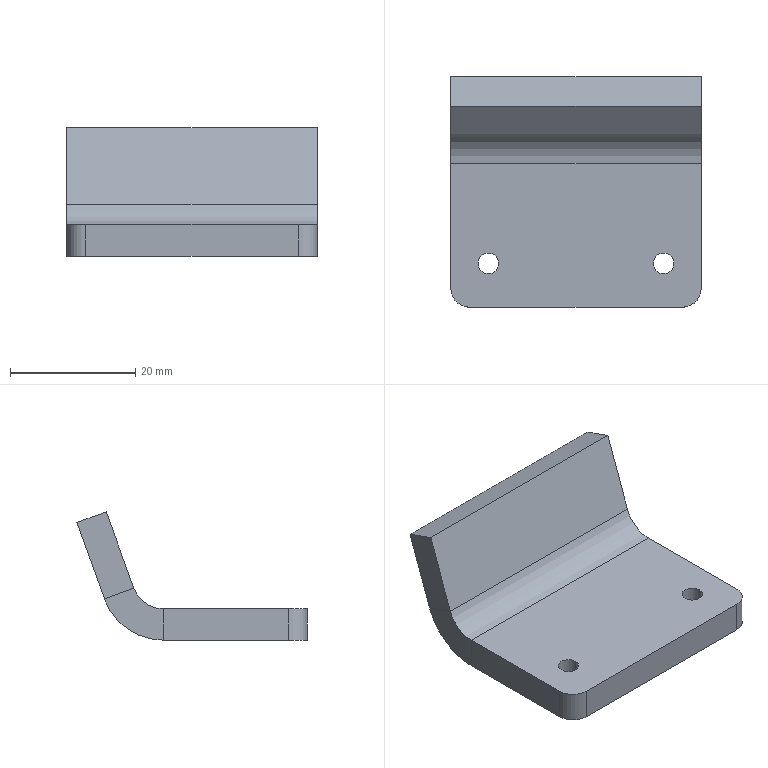Part | SolidWorks | features Fillet 1, FlatPattern 1, HoleWzd 1, ICE 1, SMBaseFlange 1, SheetMetal 1 | 1 solid | 20 faces | box 40 x 36.8 x 20.501 mm | volume 8922 mm3 | plane 12 | cylinder 8 | commonest cylinder face diameters 3.3 x4 6 x2 10 x1 20 x1
STEP:
#1=CARTESIAN_POINT('',(4.35,7.,0.));
#2=VERTEX_POINT('',#1);
#3=CARTESIAN_POINT('',(7.65,7.,0.));
#4=VERTEX_POINT('',#3);
#5=CARTESIAN_POINT('',(6.,7.,0.));
#6=DIRECTION('',(0.,0.,1.));
#7=DIRECTION('',(1.,0.,0.));
#8=AXIS2_PLACEMENT_3D('',#5,#6,#7);
#9=CIRCLE('',#8,1.65);
#10=EDGE_CURVE('',#2,#4,#9,.T.);
#11=ORIENTED_EDGE('',*,*,#10,.F.);
#12=CARTESIAN_POINT('',(4.35,7.,5.));
#13=VERTEX_POINT('',#12);
#14=CARTESIAN_POINT('',(4.35,7.,5.));
#15=DIRECTION('',(0.,0.,1.));
#16=VECTOR('',#15,1000.);
#17=LINE('',#14,#16);
#18=EDGE_CURVE('',#2,#13,#17,.T.);
#19=ORIENTED_EDGE('',*,*,#18,.T.);
#20=CARTESIAN_POINT('',(7.65,7.,5.));
#21=VERTEX_POINT('',#20);
#22=CARTESIAN_POINT('',(6.,7.,5.));
#23=DIRECTION('',(0.,0.,1.));
#24=DIRECTION('',(1.,0.,0.));
#25=AXIS2_PLACEMENT_3D('',#22,#23,#24);
#26=CIRCLE('',#25,1.65);
#27=EDGE_CURVE('',#13,#21,#26,.T.);
#28=ORIENTED_EDGE('',*,*,#27,.T.);
#29=CARTESIAN_POINT('',(7.65,7.,5.));
#30=DIRECTION('',(0.,0.,1.));
#31=VECTOR('',#30,1000.);
#32=LINE('',#29,#31);
#33=EDGE_CURVE('',#4,#21,#32,.T.);
#34=ORIENTED_EDGE('',*,*,#33,.F.);
#35=EDGE_LOOP('',(#11,#19,#28,#34));
#36=FACE_OUTER_BOUND('',#35,.T.);
#37=CARTESIAN_POINT('',(6.,7.,5.));
#38=DIRECTION('',(0.,0.,1.));
#39=DIRECTION('',(1.,0.,0.));
#40=AXIS2_PLACEMENT_3D('',#37,#38,#39);
#41=CYLINDRICAL_SURFACE('',#40,1.65);
#42=ADVANCED_FACE('',(#36),#41,.F.);
#43=CARTESIAN_POINT('',(32.35,7.,0.));
#44=VERTEX_POINT('',#43);
#45=CARTESIAN_POINT('',(35.65,7.,0.));
#46=VERTEX_POINT('',#45);
#47=CARTESIAN_POINT('',(34.,7.,0.));
#48=DIRECTION('',(0.,0.,1.));
#49=DIRECTION('',(1.,0.,0.));
#50=AXIS2_PLACEMENT_3D('',#47,#48,#49);
#51=CIRCLE('',#50,1.65);
#52=EDGE_CURVE('',#44,#46,#51,.T.);
#53=ORIENTED_EDGE('',*,*,#52,.F.);
#54=CARTESIAN_POINT('',(32.35,7.,5.));
#55=VERTEX_POINT('',#54);
#56=CARTESIAN_POINT('',(32.35,7.,5.));
#57=DIRECTION('',(0.,0.,1.));
#58=VECTOR('',#57,1000.);
#59=LINE('',#56,#58);
#60=EDGE_CURVE('',#44,#55,#59,.T.);
#61=ORIENTED_EDGE('',*,*,#60,.T.);
#62=CARTESIAN_POINT('',(35.65,7.,5.));
#63=VERTEX_POINT('',#62);
#64=CARTESIAN_POINT('',(34.,7.,5.));
#65=DIRECTION('',(0.,0.,1.));
#66=DIRECTION('',(1.,0.,0.));
#67=AXIS2_PLACEMENT_3D('',#64,#65,#66);
#68=CIRCLE('',#67,1.65);
#69=EDGE_CURVE('',#55,#63,#68,.T.);
#70=ORIENTED_EDGE('',*,*,#69,.T.);
#71=CARTESIAN_POINT('',(35.65,7.,5.));
#72=DIRECTION('',(0.,0.,1.));
#73=VECTOR('',#72,1000.);
#74=LINE('',#71,#73);
#75=EDGE_CURVE('',#46,#63,#74,.T.);
#76=ORIENTED_EDGE('',*,*,#75,.F.);
#77=EDGE_LOOP('',(#53,#61,#70,#76));
#78=FACE_OUTER_BOUND('',#77,.T.);
#79=CARTESIAN_POINT('',(34.,7.,5.));
#80=DIRECTION('',(0.,0.,1.));
#81=DIRECTION('',(1.,0.,0.));
#82=AXIS2_PLACEMENT_3D('',#79,#80,#81);
#83=CYLINDRICAL_SURFACE('',#82,1.65);
#84=ADVANCED_FACE('',(#78),#83,.F.);
#85=CARTESIAN_POINT('',(40.,22.983,0.));
#86=VERTEX_POINT('',#85);
#87=CARTESIAN_POINT('',(40.,22.983,5.));
#88=VERTEX_POINT('',#87);
#89=CARTESIAN_POINT('',(40.,22.983,0.));
#90=DIRECTION('',(0.,0.,1.));
#91=VECTOR('',#90,1000.);
#92=LINE('',#89,#91);
#93=EDGE_CURVE('',#86,#88,#92,.T.);
#94=ORIENTED_EDGE('',*,*,#93,.F.);
#95=CARTESIAN_POINT('',(40.,32.387,6.599));
#96=VERTEX_POINT('',#95);
#97=CARTESIAN_POINT('',(40.,22.983,10.));
#98=DIRECTION('',(1.,0.,0.));
#99=DIRECTION('',(0.,0.,1.));
#100=AXIS2_PLACEMENT_3D('',#97,#98,#99);
#101=CIRCLE('',#100,10.);
#102=EDGE_CURVE('',#86,#96,#101,.T.);
#103=ORIENTED_EDGE('',*,*,#102,.T.);
#104=CARTESIAN_POINT('',(40.,27.685,8.299));
#105=VERTEX_POINT('',#104);
#106=CARTESIAN_POINT('',(40.,27.685,8.299));
#107=DIRECTION('',(0.,0.9404,-0.3401));
#108=VECTOR('',#107,1000.);
#109=LINE('',#106,#108);
#110=EDGE_CURVE('',#105,#96,#109,.T.);
#111=ORIENTED_EDGE('',*,*,#110,.F.);
#112=CARTESIAN_POINT('',(40.,22.983,10.));
#113=DIRECTION('',(1.,0.,0.));
#114=DIRECTION('',(0.,0.,-1.));
#115=AXIS2_PLACEMENT_3D('',#112,#113,#114);
#116=CIRCLE('',#115,5.);
#117=EDGE_CURVE('',#88,#105,#116,.T.);
#118=ORIENTED_EDGE('',*,*,#117,.F.);
#119=EDGE_LOOP('',(#94,#103,#111,#118));
#120=FACE_OUTER_BOUND('',#119,.T.);
#121=CARTESIAN_POINT('',(40.,22.983,0.));
#122=DIRECTION('',(1.,0.,0.));
#123=DIRECTION('',(0.,0.,-1.));
#124=AXIS2_PLACEMENT_3D('',#121,#122,#123);
#125=PLANE('',#124);
#126=ADVANCED_FACE('',(#120),#125,.T.);
#127=CARTESIAN_POINT('',(40.,3.,5.));
#128=VERTEX_POINT('',#127);
#129=CARTESIAN_POINT('',(40.,0.,5.));
#130=DIRECTION('',(0.,1.,0.));
#131=VECTOR('',#130,1000.);
#132=LINE('',#129,#131);
#133=EDGE_CURVE('',#128,#88,#132,.T.);
#134=ORIENTED_EDGE('',*,*,#133,.F.);
#135=CARTESIAN_POINT('',(40.,3.,0.));
#136=VERTEX_POINT('',#135);
#137=CARTESIAN_POINT('',(40.,3.,8.299));
#138=DIRECTION('',(0.,0.,-1.));
#139=VECTOR('',#138,1000.);
#140=LINE('',#137,#139);
#141=EDGE_CURVE('',#128,#136,#140,.T.);
#142=ORIENTED_EDGE('',*,*,#141,.T.);
#143=CARTESIAN_POINT('',(40.,0.,0.));
#144=DIRECTION('',(0.,1.,0.));
#145=VECTOR('',#144,1000.);
#146=LINE('',#143,#145);
#147=EDGE_CURVE('',#136,#86,#146,.T.);
#148=ORIENTED_EDGE('',*,*,#147,.T.);
#149=ORIENTED_EDGE('',*,*,#93,.T.);
#150=EDGE_LOOP('',(#134,#142,#148,#149));
#151=FACE_OUTER_BOUND('',#150,.T.);
#152=CARTESIAN_POINT('',(40.,27.685,8.299));
#153=DIRECTION('',(1.,0.,0.));
#154=DIRECTION('',(0.,0.,-1.));
#155=AXIS2_PLACEMENT_3D('',#152,#153,#154);
#156=PLANE('',#155);
#157=ADVANCED_FACE('',(#151),#156,.T.);
#158=CARTESIAN_POINT('',(0.,32.387,6.599));
#159=VERTEX_POINT('',#158);
#160=CARTESIAN_POINT('',(0.,27.685,8.299));
#161=VERTEX_POINT('',#160);
#162=CARTESIAN_POINT('',(0.,32.387,6.599));
#163=DIRECTION('',(0.,-0.9404,0.3401));
#164=VECTOR('',#163,1000.);
#165=LINE('',#162,#164);
#166=EDGE_CURVE('',#159,#161,#165,.T.);
#167=ORIENTED_EDGE('',*,*,#166,.F.);
#168=CARTESIAN_POINT('',(0.,22.983,0.));
#169=VERTEX_POINT('',#168);
#170=CARTESIAN_POINT('',(0.,22.983,10.));
#171=DIRECTION('',(1.,0.,0.));
#172=DIRECTION('',(0.,0.,1.));
#173=AXIS2_PLACEMENT_3D('',#170,#171,#172);
#174=CIRCLE('',#173,10.);
#175=EDGE_CURVE('',#169,#159,#174,.T.);
#176=ORIENTED_EDGE('',*,*,#175,.F.);
#177=CARTESIAN_POINT('',(0.,22.983,5.));
#178=VERTEX_POINT('',#177);
#179=CARTESIAN_POINT('',(0.,22.983,5.));
#180=DIRECTION('',(0.,0.,-1.));
#181=VECTOR('',#180,1000.);
#182=LINE('',#179,#181);
#183=EDGE_CURVE('',#178,#169,#182,.T.);
#184=ORIENTED_EDGE('',*,*,#183,.F.);
#185=CARTESIAN_POINT('',(0.,22.983,10.));
#186=DIRECTION('',(1.,0.,0.));
#187=DIRECTION('',(0.,0.,-1.));
#188=AXIS2_PLACEMENT_3D('',#185,#186,#187);
#189=CIRCLE('',#188,5.);
#190=EDGE_CURVE('',#178,#161,#189,.T.);
#191=ORIENTED_EDGE('',*,*,#190,.T.);
#192=EDGE_LOOP('',(#167,#176,#184,#191));
#193=FACE_OUTER_BOUND('',#192,.T.);
#194=CARTESIAN_POINT('',(0.,32.387,6.599));
#195=DIRECTION('',(-1.,0.,0.));
#196=DIRECTION('',(0.,0.,1.));
#197=AXIS2_PLACEMENT_3D('',#194,#195,#196);
#198=PLANE('',#197);
#199=ADVANCED_FACE('',(#193),#198,.T.);
#200=CARTESIAN_POINT('',(0.,36.8,18.8));
#201=VERTEX_POINT('',#200);
#202=CARTESIAN_POINT('',(0.,30.,0.));
#203=DIRECTION('',(0.,0.3401,0.9404));
#204=VECTOR('',#203,1000.);
#205=LINE('',#202,#204);
#206=EDGE_CURVE('',#159,#201,#205,.T.);
#207=ORIENTED_EDGE('',*,*,#206,.F.);
#208=ORIENTED_EDGE('',*,*,#166,.T.);
#209=CARTESIAN_POINT('',(0.,32.098,20.501));
#210=VERTEX_POINT('',#209);
#211=CARTESIAN_POINT('',(0.,25.298,1.701));
#212=DIRECTION('',(0.,0.3401,0.9404));
#213=VECTOR('',#212,1000.);
#214=LINE('',#211,#213);
#215=EDGE_CURVE('',#161,#210,#214,.T.);
#216=ORIENTED_EDGE('',*,*,#215,.T.);
#217=CARTESIAN_POINT('',(0.,32.098,20.501));
#218=DIRECTION('',(0.,0.9404,-0.3401));
#219=VECTOR('',#218,1000.);
#220=LINE('',#217,#219);
#221=EDGE_CURVE('',#210,#201,#220,.T.);
#222=ORIENTED_EDGE('',*,*,#221,.T.);
#223=EDGE_LOOP('',(#207,#208,#216,#222));
#224=FACE_OUTER_BOUND('',#223,.T.);
#225=CARTESIAN_POINT('',(0.,22.983,5.));
#226=DIRECTION('',(-1.,0.,0.));
#227=DIRECTION('',(0.,0.,1.));
#228=AXIS2_PLACEMENT_3D('',#225,#226,#227);
#229=PLANE('',#228);
#230=ADVANCED_FACE('',(#224),#229,.T.);
#231=ORIENTED_EDGE('',*,*,#206,.T.);
#232=CARTESIAN_POINT('',(40.,36.8,18.8));
#233=VERTEX_POINT('',#232);
#234=CARTESIAN_POINT('',(40.,36.8,18.8));
#235=DIRECTION('',(-1.,0.,0.));
#236=VECTOR('',#235,1000.);
#237=LINE('',#234,#236);
#238=EDGE_CURVE('',#233,#201,#237,.T.);
#239=ORIENTED_EDGE('',*,*,#238,.F.);
#240=CARTESIAN_POINT('',(40.,30.,0.));
#241=DIRECTION('',(0.,0.3401,0.9404));
#242=VECTOR('',#241,1000.);
#243=LINE('',#240,#242);
#244=EDGE_CURVE('',#96,#233,#243,.T.);
#245=ORIENTED_EDGE('',*,*,#244,.F.);
#246=CARTESIAN_POINT('',(40.,32.387,6.599));
#247=DIRECTION('',(-1.,0.,0.));
#248=VECTOR('',#247,1000.);
#249=LINE('',#246,#248);
#250=EDGE_CURVE('',#96,#159,#249,.T.);
#251=ORIENTED_EDGE('',*,*,#250,.T.);
#252=EDGE_LOOP('',(#231,#239,#245,#251));
#253=FACE_OUTER_BOUND('',#252,.T.);
#254=CARTESIAN_POINT('',(40.,30.,0.));
#255=DIRECTION('',(0.,-0.9404,0.3401));
#256=DIRECTION('',(0.,-0.3401,-0.9404));
#257=AXIS2_PLACEMENT_3D('',#254,#255,#256);
#258=PLANE('',#257);
#259=ADVANCED_FACE('',(#253),#258,.F.);
#260=ORIENTED_EDGE('',*,*,#221,.F.);
#261=CARTESIAN_POINT('',(40.,32.098,20.501));
#262=VERTEX_POINT('',#261);
#263=CARTESIAN_POINT('',(40.,32.098,20.501));
#264=DIRECTION('',(-1.,0.,0.));
#265=VECTOR('',#264,1000.);
#266=LINE('',#263,#265);
#267=EDGE_CURVE('',#262,#210,#266,.T.);
#268=ORIENTED_EDGE('',*,*,#267,.F.);
#269=CARTESIAN_POINT('',(40.,32.098,20.501));
#270=DIRECTION('',(0.,0.9404,-0.3401));
#271=VECTOR('',#270,1000.);
#272=LINE('',#269,#271);
#273=EDGE_CURVE('',#262,#233,#272,.T.);
#274=ORIENTED_EDGE('',*,*,#273,.T.);
#275=ORIENTED_EDGE('',*,*,#238,.T.);
#276=EDGE_LOOP('',(#260,#268,#274,#275));
#277=FACE_OUTER_BOUND('',#276,.T.);
#278=CARTESIAN_POINT('',(40.,32.098,20.501));
#279=DIRECTION('',(0.,0.3401,0.9404));
#280=DIRECTION('',(0.,-0.9404,0.3401));
#281=AXIS2_PLACEMENT_3D('',#278,#279,#280);
#282=PLANE('',#281);
#283=ADVANCED_FACE('',(#277),#282,.T.);
#284=ORIENTED_EDGE('',*,*,#215,.F.);
#285=CARTESIAN_POINT('',(40.,27.685,8.299));
#286=DIRECTION('',(-1.,0.,0.));
#287=VECTOR('',#286,1000.);
#288=LINE('',#285,#287);
#289=EDGE_CURVE('',#105,#161,#288,.T.);
#290=ORIENTED_EDGE('',*,*,#289,.F.);
#291=CARTESIAN_POINT('',(40.,25.298,1.701));
#292=DIRECTION('',(0.,0.3401,0.9404));
#293=VECTOR('',#292,1000.);
#294=LINE('',#291,#293);
#295=EDGE_CURVE('',#105,#262,#294,.T.);
#296=ORIENTED_EDGE('',*,*,#295,.T.);
#297=ORIENTED_EDGE('',*,*,#267,.T.);
#298=EDGE_LOOP('',(#284,#290,#296,#297));
#299=FACE_OUTER_BOUND('',#298,.T.);
#300=CARTESIAN_POINT('',(40.,25.298,1.701));
#301=DIRECTION('',(0.,-0.9404,0.3401));
#302=DIRECTION('',(0.,-0.3401,-0.9404));
#303=AXIS2_PLACEMENT_3D('',#300,#301,#302);
#304=PLANE('',#303);
#305=ADVANCED_FACE('',(#299),#304,.T.);
#306=ORIENTED_EDGE('',*,*,#190,.F.);
#307=CARTESIAN_POINT('',(40.,22.983,5.));
#308=DIRECTION('',(-1.,0.,0.));
#309=VECTOR('',#308,1000.);
#310=LINE('',#307,#309);
#311=EDGE_CURVE('',#88,#178,#310,.T.);
#312=ORIENTED_EDGE('',*,*,#311,.F.);
#313=ORIENTED_EDGE('',*,*,#117,.T.);
#314=ORIENTED_EDGE('',*,*,#289,.T.);
#315=EDGE_LOOP('',(#306,#312,#313,#314));
#316=FACE_OUTER_BOUND('',#315,.T.);
#317=CARTESIAN_POINT('',(40.,22.983,10.));
#318=DIRECTION('',(-1.,0.,0.));
#319=DIRECTION('',(0.,0.,1.));
#320=AXIS2_PLACEMENT_3D('',#317,#318,#319);
#321=CYLINDRICAL_SURFACE('',#320,5.);
#322=ADVANCED_FACE('',(#316),#321,.F.);
#323=CARTESIAN_POINT('',(6.,7.,5.));
#324=DIRECTION('',(0.,0.,1.));
#325=DIRECTION('',(1.,0.,0.));
#326=AXIS2_PLACEMENT_3D('',#323,#324,#325);
#327=CIRCLE('',#326,1.65);
#328=EDGE_CURVE('',#21,#13,#327,.T.);
#329=ORIENTED_EDGE('',*,*,#328,.F.);
#330=ORIENTED_EDGE('',*,*,#27,.F.);
#331=EDGE_LOOP('',(#329,#330));
#332=FACE_BOUND('',#331,.T.);
#333=CARTESIAN_POINT('',(34.,7.,5.));
#334=DIRECTION('',(0.,0.,1.));
#335=DIRECTION('',(1.,0.,0.));
#336=AXIS2_PLACEMENT_3D('',#333,#334,#335);
#337=CIRCLE('',#336,1.65);
#338=EDGE_CURVE('',#63,#55,#337,.T.);
#339=ORIENTED_EDGE('',*,*,#338,.F.);
#340=ORIENTED_EDGE('',*,*,#69,.F.);
#341=EDGE_LOOP('',(#339,#340));
#342=FACE_BOUND('',#341,.T.);
#343=CARTESIAN_POINT('',(37.,0.,5.));
#344=VERTEX_POINT('',#343);
#345=CARTESIAN_POINT('',(3.,0.,5.));
#346=VERTEX_POINT('',#345);
#347=CARTESIAN_POINT('',(40.,0.,5.));
#348=DIRECTION('',(-1.,0.,0.));
#349=VECTOR('',#348,1000.);
#350=LINE('',#347,#349);
#351=EDGE_CURVE('',#344,#346,#350,.T.);
#352=ORIENTED_EDGE('',*,*,#351,.F.);
#353=CARTESIAN_POINT('',(37.,3.,5.));
#354=DIRECTION('',(0.,0.,1.));
#355=DIRECTION('',(1.,0.,0.));
#356=AXIS2_PLACEMENT_3D('',#353,#354,#355);
#357=CIRCLE('',#356,3.);
#358=EDGE_CURVE('',#344,#128,#357,.T.);
#359=ORIENTED_EDGE('',*,*,#358,.T.);
#360=ORIENTED_EDGE('',*,*,#133,.T.);
#361=ORIENTED_EDGE('',*,*,#311,.T.);
#362=CARTESIAN_POINT('',(0.,3.,5.));
#363=VERTEX_POINT('',#362);
#364=CARTESIAN_POINT('',(0.,0.,5.));
#365=DIRECTION('',(0.,1.,0.));
#366=VECTOR('',#365,1000.);
#367=LINE('',#364,#366);
#368=EDGE_CURVE('',#363,#178,#367,.T.);
#369=ORIENTED_EDGE('',*,*,#368,.F.);
#370=CARTESIAN_POINT('',(3.,3.,5.));
#371=DIRECTION('',(0.,0.,1.));
#372=DIRECTION('',(1.,0.,0.));
#373=AXIS2_PLACEMENT_3D('',#370,#371,#372);
#374=CIRCLE('',#373,3.);
#375=EDGE_CURVE('',#363,#346,#374,.T.);
#376=ORIENTED_EDGE('',*,*,#375,.T.);
#377=EDGE_LOOP('',(#352,#359,#360,#361,#369,#376));
#378=FACE_OUTER_BOUND('',#377,.T.);
#379=CARTESIAN_POINT('',(40.,0.,5.));
#380=DIRECTION('',(0.,0.,1.));
#381=DIRECTION('',(1.,0.,0.));
#382=AXIS2_PLACEMENT_3D('',#379,#380,#381);
#383=PLANE('',#382);
#384=ADVANCED_FACE('',(#332,#342,#378),#383,.T.);
#385=CARTESIAN_POINT('',(37.,0.,0.));
#386=VERTEX_POINT('',#385);
#387=CARTESIAN_POINT('',(3.,0.,0.));
#388=VERTEX_POINT('',#387);
#389=CARTESIAN_POINT('',(40.,0.,0.));
#390=DIRECTION('',(-1.,0.,0.));
#391=VECTOR('',#390,1000.);
#392=LINE('',#389,#391);
#393=EDGE_CURVE('',#386,#388,#392,.T.);
#394=ORIENTED_EDGE('',*,*,#393,.F.);
#395=CARTESIAN_POINT('',(37.,0.,0.));
#396=DIRECTION('',(0.,0.,1.));
#397=VECTOR('',#396,1000.);
#398=LINE('',#395,#397);
#399=EDGE_CURVE('',#386,#344,#398,.T.);
#400=ORIENTED_EDGE('',*,*,#399,.T.);
#401=ORIENTED_EDGE('',*,*,#351,.T.);
#402=CARTESIAN_POINT('',(3.,0.,0.));
#403=DIRECTION('',(0.,0.,-1.));
#404=VECTOR('',#403,1000.);
#405=LINE('',#402,#404);
#406=EDGE_CURVE('',#346,#388,#405,.T.);
#407=ORIENTED_EDGE('',*,*,#406,.T.);
#408=EDGE_LOOP('',(#394,#400,#401,#407));
#409=FACE_OUTER_BOUND('',#408,.T.);
#410=CARTESIAN_POINT('',(40.,0.,0.));
#411=DIRECTION('',(0.,-1.,0.));
#412=DIRECTION('',(0.,0.,-1.));
#413=AXIS2_PLACEMENT_3D('',#410,#411,#412);
#414=PLANE('',#413);
#415=ADVANCED_FACE('',(#409),#414,.T.);
#416=CARTESIAN_POINT('',(6.,7.,0.));
#417=DIRECTION('',(0.,0.,1.));
#418=DIRECTION('',(1.,0.,0.));
#419=AXIS2_PLACEMENT_3D('',#416,#417,#418);
#420=CIRCLE('',#419,1.65);
#421=EDGE_CURVE('',#4,#2,#420,.T.);
#422=ORIENTED_EDGE('',*,*,#421,.T.);
#423=ORIENTED_EDGE('',*,*,#10,.T.);
#424=EDGE_LOOP('',(#422,#423));
#425=FACE_BOUND('',#424,.T.);
#426=CARTESIAN_POINT('',(34.,7.,0.));
#427=DIRECTION('',(0.,0.,1.));
#428=DIRECTION('',(1.,0.,0.));
#429=AXIS2_PLACEMENT_3D('',#426,#427,#428);
#430=CIRCLE('',#429,1.65);
#431=EDGE_CURVE('',#46,#44,#430,.T.);
#432=ORIENTED_EDGE('',*,*,#431,.T.);
#433=ORIENTED_EDGE('',*,*,#52,.T.);
#434=EDGE_LOOP('',(#432,#433));
#435=FACE_BOUND('',#434,.T.);
#436=ORIENTED_EDGE('',*,*,#147,.F.);
#437=CARTESIAN_POINT('',(37.,3.,0.));
#438=DIRECTION('',(0.,0.,-1.));
#439=DIRECTION('',(1.,0.,0.));
#440=AXIS2_PLACEMENT_3D('',#437,#438,#439);
#441=CIRCLE('',#440,3.);
#442=EDGE_CURVE('',#136,#386,#441,.T.);
#443=ORIENTED_EDGE('',*,*,#442,.T.);
#444=ORIENTED_EDGE('',*,*,#393,.T.);
#445=CARTESIAN_POINT('',(0.,3.,0.));
#446=VERTEX_POINT('',#445);
#447=CARTESIAN_POINT('',(3.,3.,0.));
#448=DIRECTION('',(0.,0.,-1.));
#449=DIRECTION('',(1.,0.,0.));
#450=AXIS2_PLACEMENT_3D('',#447,#448,#449);
#451=CIRCLE('',#450,3.);
#452=EDGE_CURVE('',#388,#446,#451,.T.);
#453=ORIENTED_EDGE('',*,*,#452,.T.);
#454=CARTESIAN_POINT('',(0.,0.,0.));
#455=DIRECTION('',(0.,1.,0.));
#456=VECTOR('',#455,1000.);
#457=LINE('',#454,#456);
#458=EDGE_CURVE('',#446,#169,#457,.T.);
#459=ORIENTED_EDGE('',*,*,#458,.T.);
#460=CARTESIAN_POINT('',(40.,22.983,0.));
#461=DIRECTION('',(-1.,0.,0.));
#462=VECTOR('',#461,1000.);
#463=LINE('',#460,#462);
#464=EDGE_CURVE('',#86,#169,#463,.T.);
#465=ORIENTED_EDGE('',*,*,#464,.F.);
#466=EDGE_LOOP('',(#436,#443,#444,#453,#459,#465));
#467=FACE_OUTER_BOUND('',#466,.T.);
#468=CARTESIAN_POINT('',(40.,0.,0.));
#469=DIRECTION('',(0.,0.,1.));
#470=DIRECTION('',(1.,0.,0.));
#471=AXIS2_PLACEMENT_3D('',#468,#469,#470);
#472=PLANE('',#471);
#473=ADVANCED_FACE('',(#425,#435,#467),#472,.F.);
#474=ORIENTED_EDGE('',*,*,#175,.T.);
#475=ORIENTED_EDGE('',*,*,#250,.F.);
#476=ORIENTED_EDGE('',*,*,#102,.F.);
#477=ORIENTED_EDGE('',*,*,#464,.T.);
#478=EDGE_LOOP('',(#474,#475,#476,#477));
#479=FACE_OUTER_BOUND('',#478,.T.);
#480=CARTESIAN_POINT('',(40.,22.983,10.));
#481=DIRECTION('',(-1.,0.,0.));
#482=DIRECTION('',(0.,0.,1.));
#483=AXIS2_PLACEMENT_3D('',#480,#481,#482);
#484=CYLINDRICAL_SURFACE('',#483,10.);
#485=ADVANCED_FACE('',(#479),#484,.T.);
#486=ORIENTED_EDGE('',*,*,#244,.T.);
#487=ORIENTED_EDGE('',*,*,#273,.F.);
#488=ORIENTED_EDGE('',*,*,#295,.F.);
#489=ORIENTED_EDGE('',*,*,#110,.T.);
#490=EDGE_LOOP('',(#486,#487,#488,#489));
#491=FACE_OUTER_BOUND('',#490,.T.);
#492=CARTESIAN_POINT('',(40.,22.983,10.));
#493=DIRECTION('',(1.,0.,0.));
#494=DIRECTION('',(0.,0.,-1.));
#495=AXIS2_PLACEMENT_3D('',#492,#493,#494);
#496=PLANE('',#495);
#497=ADVANCED_FACE('',(#491),#496,.T.);
#498=ORIENTED_EDGE('',*,*,#458,.F.);
#499=CARTESIAN_POINT('',(0.,3.,5.));
#500=DIRECTION('',(0.,0.,1.));
#501=VECTOR('',#500,1000.);
#502=LINE('',#499,#501);
#503=EDGE_CURVE('',#446,#363,#502,.T.);
#504=ORIENTED_EDGE('',*,*,#503,.T.);
#505=ORIENTED_EDGE('',*,*,#368,.T.);
#506=ORIENTED_EDGE('',*,*,#183,.T.);
#507=EDGE_LOOP('',(#498,#504,#505,#506));
#508=FACE_OUTER_BOUND('',#507,.T.);
#509=CARTESIAN_POINT('',(0.,22.983,10.));
#510=DIRECTION('',(1.,0.,0.));
#511=DIRECTION('',(0.,0.,-1.));
#512=AXIS2_PLACEMENT_3D('',#509,#510,#511);
#513=PLANE('',#512);
#514=ADVANCED_FACE('',(#508),#513,.F.);
#515=ORIENTED_EDGE('',*,*,#60,.F.);
#516=ORIENTED_EDGE('',*,*,#431,.F.);
#517=ORIENTED_EDGE('',*,*,#75,.T.);
#518=ORIENTED_EDGE('',*,*,#338,.T.);
#519=EDGE_LOOP('',(#515,#516,#517,#518));
#520=FACE_OUTER_BOUND('',#519,.T.);
#521=CARTESIAN_POINT('',(34.,7.,5.));
#522=DIRECTION('',(0.,0.,1.));
#523=DIRECTION('',(1.,0.,0.));
#524=AXIS2_PLACEMENT_3D('',#521,#522,#523);
#525=CYLINDRICAL_SURFACE('',#524,1.65);
#526=ADVANCED_FACE('',(#520),#525,.F.);
#527=ORIENTED_EDGE('',*,*,#18,.F.);
#528=ORIENTED_EDGE('',*,*,#421,.F.);
#529=ORIENTED_EDGE('',*,*,#33,.T.);
#530=ORIENTED_EDGE('',*,*,#328,.T.);
#531=EDGE_LOOP('',(#527,#528,#529,#530));
#532=FACE_OUTER_BOUND('',#531,.T.);
#533=CARTESIAN_POINT('',(6.,7.,5.));
#534=DIRECTION('',(0.,0.,1.));
#535=DIRECTION('',(1.,0.,0.));
#536=AXIS2_PLACEMENT_3D('',#533,#534,#535);
#537=CYLINDRICAL_SURFACE('',#536,1.65);
#538=ADVANCED_FACE('',(#532),#537,.F.);
#539=ORIENTED_EDGE('',*,*,#442,.F.);
#540=ORIENTED_EDGE('',*,*,#141,.F.);
#541=ORIENTED_EDGE('',*,*,#358,.F.);
#542=ORIENTED_EDGE('',*,*,#399,.F.);
#543=EDGE_LOOP('',(#539,#540,#541,#542));
#544=FACE_OUTER_BOUND('',#543,.T.);
#545=CARTESIAN_POINT('',(37.,3.,0.));
#546=DIRECTION('',(0.,0.,1.));
#547=DIRECTION('',(1.,0.,0.));
#548=AXIS2_PLACEMENT_3D('',#545,#546,#547);
#549=CYLINDRICAL_SURFACE('',#548,3.);
#550=ADVANCED_FACE('',(#544),#549,.T.);
#551=ORIENTED_EDGE('',*,*,#452,.F.);
#552=ORIENTED_EDGE('',*,*,#406,.F.);
#553=ORIENTED_EDGE('',*,*,#375,.F.);
#554=ORIENTED_EDGE('',*,*,#503,.F.);
#555=EDGE_LOOP('',(#551,#552,#553,#554));
#556=FACE_OUTER_BOUND('',#555,.T.);
#557=CARTESIAN_POINT('',(3.,3.,10.));
#558=DIRECTION('',(0.,0.,-1.));
#559=DIRECTION('',(-1.,0.,0.));
#560=AXIS2_PLACEMENT_3D('',#557,#558,#559);
#561=CYLINDRICAL_SURFACE('',#560,3.);
#562=ADVANCED_FACE('',(#556),#561,.T.);
#563=CLOSED_SHELL('',(#42,#84,#126,#157,#199,#230,#259,#283,#305,#322,#384,#415,#473,#485,#497,#514,#526,#538,#550,#562));
#564=MANIFOLD_SOLID_BREP('',#563);
#565=CARTESIAN_POINT('',(0.,0.,0.));
#566=DIRECTION('',(0.,0.,1.));
#567=DIRECTION('',(1.,0.,0.));
#568=AXIS2_PLACEMENT_3D('',#565,#566,#567);
#569=(LENGTH_UNIT()NAMED_UNIT(*)SI_UNIT(.MILLI.,.METRE.));
#570=UNCERTAINTY_MEASURE_WITH_UNIT(LENGTH_MEASURE(0.00001),#569,'','');
#571=(NAMED_UNIT(*)PLANE_ANGLE_UNIT()SI_UNIT($,.RADIAN.));
#572=(NAMED_UNIT(*)SI_UNIT($,.STERADIAN.)SOLID_ANGLE_UNIT());
#573=(GEOMETRIC_REPRESENTATION_CONTEXT(3)GLOBAL_UNCERTAINTY_ASSIGNED_CONTEXT((#570))GLOBAL_UNIT_ASSIGNED_CONTEXT((#569,#571,#572))REPRESENTATION_CONTEXT('',''));
#574=ADVANCED_BREP_SHAPE_REPRESENTATION('',(#564,#568),#573);